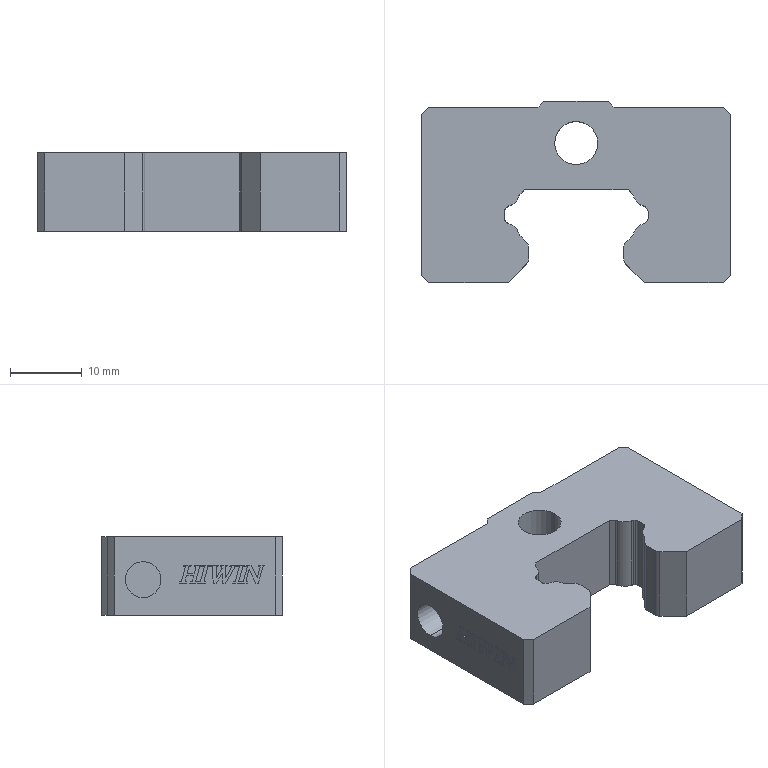Part | STEP file | PART2A^SUB1AA_P-008243 | 1 solid | 206 faces | box 43 x 25.2 x 11 mm | volume 8694 mm3 | plane 143 | cylinder 63 | commonest cylinder face diameters 0.2 x17 1 x16 0.1 x9 2 x4 4.06 x4 5 x4